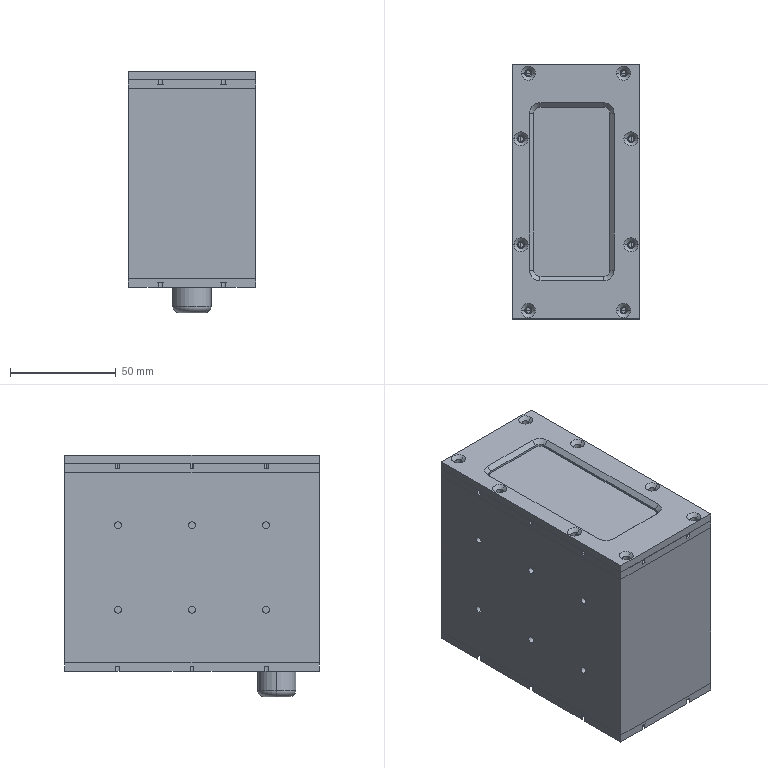Part | 13 solids | 415 faces | box 60 x 120 x 114 mm | volume 214263 mm3 | cylinder 234 | plane 109 | cone 68 | torus 4 | commonest cylinder face diameters 4.4 x42 1.6 x40 2.4 x40 2.5 x32 3.3 x24 3.4 x24